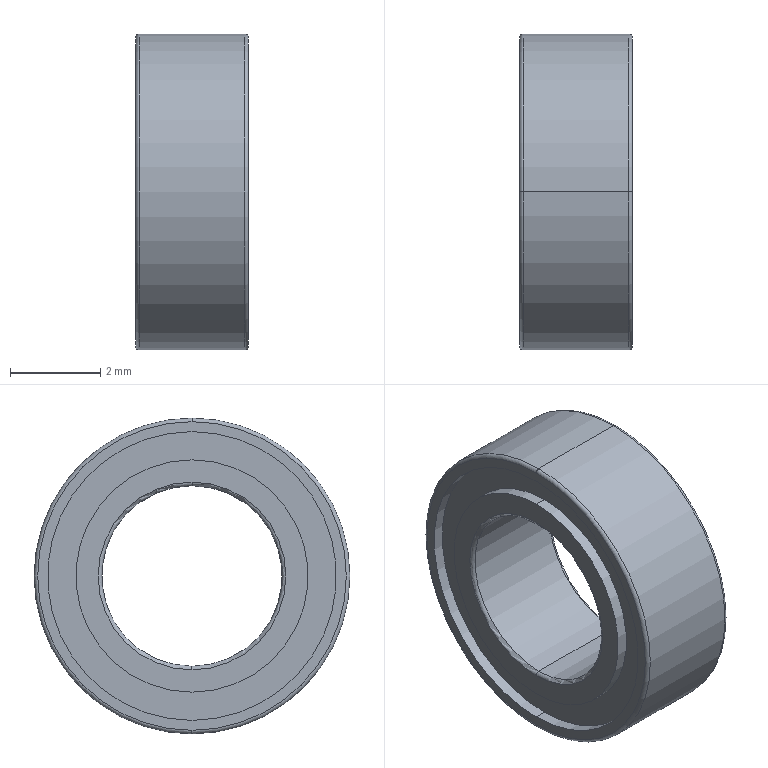Part | SolidWorks | features RefAxis 6, 3DProfileFeature 2, Revolution 1 | 1 solid | 26 faces | box 2.5 x 7 x 7 mm | volume 58.917 mm3 | cylinder 12 | torus 8 | plane 6 | commonest cylinder face diameters 5.15 x4 6.4 x4 4 x2 7 x2
STEP:
#1=CARTESIAN_POINT('',(2.42,0.,3.5));
#2=VERTEX_POINT('',#1);
#3=CARTESIAN_POINT('',(2.42,0.,-3.5));
#4=VERTEX_POINT('',#3);
#5=CARTESIAN_POINT('',(2.42,0.,0.));
#6=DIRECTION('',(-1.,0.,0.));
#7=DIRECTION('',(0.,0.,1.));
#8=AXIS2_PLACEMENT_3D('',#5,#6,#7);
#9=CIRCLE('',#8,3.5);
#10=EDGE_CURVE('',#2,#4,#9,.T.);
#11=ORIENTED_EDGE('',*,*,#10,.T.);
#12=CARTESIAN_POINT('',(0.08,0.,-3.5));
#13=VERTEX_POINT('',#12);
#14=CARTESIAN_POINT('',(2.42,0.,-3.5));
#15=DIRECTION('',(-1.,0.,0.));
#16=VECTOR('',#15,1000.);
#17=LINE('',#14,#16);
#18=EDGE_CURVE('',#4,#13,#17,.T.);
#19=ORIENTED_EDGE('',*,*,#18,.T.);
#20=CARTESIAN_POINT('',(0.08,0.,3.5));
#21=VERTEX_POINT('',#20);
#22=CARTESIAN_POINT('',(0.08,0.,0.));
#23=DIRECTION('',(-1.,0.,0.));
#24=DIRECTION('',(0.,0.,1.));
#25=AXIS2_PLACEMENT_3D('',#22,#23,#24);
#26=CIRCLE('',#25,3.5);
#27=EDGE_CURVE('',#21,#13,#26,.T.);
#28=ORIENTED_EDGE('',*,*,#27,.F.);
#29=CARTESIAN_POINT('',(2.42,0.,3.5));
#30=DIRECTION('',(-1.,0.,0.));
#31=VECTOR('',#30,1000.);
#32=LINE('',#29,#31);
#33=EDGE_CURVE('',#2,#21,#32,.T.);
#34=ORIENTED_EDGE('',*,*,#33,.F.);
#35=EDGE_LOOP('',(#11,#19,#28,#34));
#36=FACE_OUTER_BOUND('',#35,.T.);
#37=CARTESIAN_POINT('',(2.42,0.,0.));
#38=DIRECTION('',(-1.,0.,0.));
#39=DIRECTION('',(0.,0.,1.));
#40=AXIS2_PLACEMENT_3D('',#37,#38,#39);
#41=CYLINDRICAL_SURFACE('',#40,3.5);
#42=ADVANCED_FACE('',(#36),#41,.T.);
#43=CARTESIAN_POINT('',(2.5,0.,3.42));
#44=VERTEX_POINT('',#43);
#45=CARTESIAN_POINT('',(2.5,0.,-3.42));
#46=VERTEX_POINT('',#45);
#47=CARTESIAN_POINT('',(2.5,0.,0.));
#48=DIRECTION('',(-1.,0.,0.));
#49=DIRECTION('',(0.,0.,1.));
#50=AXIS2_PLACEMENT_3D('',#47,#48,#49);
#51=CIRCLE('',#50,3.42);
#52=EDGE_CURVE('',#44,#46,#51,.T.);
#53=ORIENTED_EDGE('',*,*,#52,.T.);
#54=CARTESIAN_POINT('',(2.42,0.,-3.42));
#55=DIRECTION('',(0.,1.,0.));
#56=DIRECTION('',(0.,0.,1.));
#57=AXIS2_PLACEMENT_3D('',#54,#55,#56);
#58=CIRCLE('',#57,0.08);
#59=EDGE_CURVE('',#46,#4,#58,.T.);
#60=ORIENTED_EDGE('',*,*,#59,.T.);
#61=ORIENTED_EDGE('',*,*,#10,.F.);
#62=CARTESIAN_POINT('',(2.42,0.,3.42));
#63=DIRECTION('',(0.,-1.,0.));
#64=DIRECTION('',(0.,0.,-1.));
#65=AXIS2_PLACEMENT_3D('',#62,#63,#64);
#66=CIRCLE('',#65,0.08);
#67=EDGE_CURVE('',#44,#2,#66,.T.);
#68=ORIENTED_EDGE('',*,*,#67,.F.);
#69=EDGE_LOOP('',(#53,#60,#61,#68));
#70=FACE_OUTER_BOUND('',#69,.T.);
#71=CARTESIAN_POINT('',(2.42,0.,0.));
#72=DIRECTION('',(-1.,0.,0.));
#73=DIRECTION('',(0.,0.,1.));
#74=AXIS2_PLACEMENT_3D('',#71,#72,#73);
#75=TOROIDAL_SURFACE('',#74,3.42,0.08);
#76=ADVANCED_FACE('',(#70),#75,.T.);
#77=CARTESIAN_POINT('',(2.5,0.,-3.2));
#78=VERTEX_POINT('',#77);
#79=CARTESIAN_POINT('',(2.5,0.,3.2));
#80=VERTEX_POINT('',#79);
#81=CARTESIAN_POINT('',(2.5,0.,0.));
#82=DIRECTION('',(-1.,0.,0.));
#83=DIRECTION('',(0.,0.,1.));
#84=AXIS2_PLACEMENT_3D('',#81,#82,#83);
#85=CIRCLE('',#84,3.2);
#86=EDGE_CURVE('',#78,#80,#85,.T.);
#87=ORIENTED_EDGE('',*,*,#86,.F.);
#88=CARTESIAN_POINT('',(2.245,0.,-3.2));
#89=VERTEX_POINT('',#88);
#90=CARTESIAN_POINT('',(2.42,0.,-3.2));
#91=DIRECTION('',(-1.,0.,0.));
#92=VECTOR('',#91,1000.);
#93=LINE('',#90,#92);
#94=EDGE_CURVE('',#78,#89,#93,.T.);
#95=ORIENTED_EDGE('',*,*,#94,.T.);
#96=CARTESIAN_POINT('',(2.245,0.,3.2));
#97=VERTEX_POINT('',#96);
#98=CARTESIAN_POINT('',(2.245,0.,0.));
#99=DIRECTION('',(-1.,0.,0.));
#100=DIRECTION('',(0.,0.,1.));
#101=AXIS2_PLACEMENT_3D('',#98,#99,#100);
#102=CIRCLE('',#101,3.2);
#103=EDGE_CURVE('',#89,#97,#102,.T.);
#104=ORIENTED_EDGE('',*,*,#103,.T.);
#105=CARTESIAN_POINT('',(2.42,0.,3.2));
#106=DIRECTION('',(-1.,0.,0.));
#107=VECTOR('',#106,1000.);
#108=LINE('',#105,#107);
#109=EDGE_CURVE('',#80,#97,#108,.T.);
#110=ORIENTED_EDGE('',*,*,#109,.F.);
#111=EDGE_LOOP('',(#87,#95,#104,#110));
#112=FACE_OUTER_BOUND('',#111,.T.);
#113=CARTESIAN_POINT('',(2.42,0.,0.));
#114=DIRECTION('',(-1.,0.,0.));
#115=DIRECTION('',(0.,0.,1.));
#116=AXIS2_PLACEMENT_3D('',#113,#114,#115);
#117=CYLINDRICAL_SURFACE('',#116,3.2);
#118=ADVANCED_FACE('',(#112),#117,.F.);
#119=CARTESIAN_POINT('',(2.5,0.,2.575));
#120=VERTEX_POINT('',#119);
#121=CARTESIAN_POINT('',(2.5,0.,-2.575));
#122=VERTEX_POINT('',#121);
#123=CARTESIAN_POINT('',(2.5,0.,0.));
#124=DIRECTION('',(-1.,0.,0.));
#125=DIRECTION('',(0.,0.,1.));
#126=AXIS2_PLACEMENT_3D('',#123,#124,#125);
#127=CIRCLE('',#126,2.575);
#128=EDGE_CURVE('',#120,#122,#127,.T.);
#129=ORIENTED_EDGE('',*,*,#128,.T.);
#130=CARTESIAN_POINT('',(2.245,0.,-2.575));
#131=VERTEX_POINT('',#130);
#132=CARTESIAN_POINT('',(2.42,0.,-2.575));
#133=DIRECTION('',(-1.,0.,0.));
#134=VECTOR('',#133,1000.);
#135=LINE('',#132,#134);
#136=EDGE_CURVE('',#122,#131,#135,.T.);
#137=ORIENTED_EDGE('',*,*,#136,.T.);
#138=CARTESIAN_POINT('',(2.245,0.,2.575));
#139=VERTEX_POINT('',#138);
#140=CARTESIAN_POINT('',(2.245,0.,0.));
#141=DIRECTION('',(-1.,0.,0.));
#142=DIRECTION('',(0.,0.,1.));
#143=AXIS2_PLACEMENT_3D('',#140,#141,#142);
#144=CIRCLE('',#143,2.575);
#145=EDGE_CURVE('',#139,#131,#144,.T.);
#146=ORIENTED_EDGE('',*,*,#145,.F.);
#147=CARTESIAN_POINT('',(2.42,0.,2.575));
#148=DIRECTION('',(-1.,0.,0.));
#149=VECTOR('',#148,1000.);
#150=LINE('',#147,#149);
#151=EDGE_CURVE('',#120,#139,#150,.T.);
#152=ORIENTED_EDGE('',*,*,#151,.F.);
#153=EDGE_LOOP('',(#129,#137,#146,#152));
#154=FACE_OUTER_BOUND('',#153,.T.);
#155=CARTESIAN_POINT('',(2.42,0.,0.));
#156=DIRECTION('',(-1.,0.,0.));
#157=DIRECTION('',(0.,0.,1.));
#158=AXIS2_PLACEMENT_3D('',#155,#156,#157);
#159=CYLINDRICAL_SURFACE('',#158,2.575);
#160=ADVANCED_FACE('',(#154),#159,.T.);
#161=CARTESIAN_POINT('',(2.42,0.,2.));
#162=VERTEX_POINT('',#161);
#163=CARTESIAN_POINT('',(2.42,0.,-2.));
#164=VERTEX_POINT('',#163);
#165=CARTESIAN_POINT('',(2.42,0.,0.));
#166=DIRECTION('',(-1.,0.,0.));
#167=DIRECTION('',(0.,0.,1.));
#168=AXIS2_PLACEMENT_3D('',#165,#166,#167);
#169=CIRCLE('',#168,2.);
#170=EDGE_CURVE('',#162,#164,#169,.T.);
#171=ORIENTED_EDGE('',*,*,#170,.T.);
#172=CARTESIAN_POINT('',(2.5,0.,-2.08));
#173=VERTEX_POINT('',#172);
#174=CARTESIAN_POINT('',(2.42,0.,-2.08));
#175=DIRECTION('',(0.,1.,0.));
#176=DIRECTION('',(0.,0.,1.));
#177=AXIS2_PLACEMENT_3D('',#174,#175,#176);
#178=CIRCLE('',#177,0.08);
#179=EDGE_CURVE('',#164,#173,#178,.T.);
#180=ORIENTED_EDGE('',*,*,#179,.T.);
#181=CARTESIAN_POINT('',(2.5,0.,2.08));
#182=VERTEX_POINT('',#181);
#183=CARTESIAN_POINT('',(2.5,0.,0.));
#184=DIRECTION('',(-1.,0.,0.));
#185=DIRECTION('',(0.,0.,1.));
#186=AXIS2_PLACEMENT_3D('',#183,#184,#185);
#187=CIRCLE('',#186,2.08);
#188=EDGE_CURVE('',#182,#173,#187,.T.);
#189=ORIENTED_EDGE('',*,*,#188,.F.);
#190=CARTESIAN_POINT('',(2.42,0.,2.08));
#191=DIRECTION('',(0.,-1.,0.));
#192=DIRECTION('',(0.,0.,-1.));
#193=AXIS2_PLACEMENT_3D('',#190,#191,#192);
#194=CIRCLE('',#193,0.08);
#195=EDGE_CURVE('',#162,#182,#194,.T.);
#196=ORIENTED_EDGE('',*,*,#195,.F.);
#197=EDGE_LOOP('',(#171,#180,#189,#196));
#198=FACE_OUTER_BOUND('',#197,.T.);
#199=CARTESIAN_POINT('',(2.42,0.,0.));
#200=DIRECTION('',(-1.,0.,0.));
#201=DIRECTION('',(0.,0.,1.));
#202=AXIS2_PLACEMENT_3D('',#199,#200,#201);
#203=TOROIDAL_SURFACE('',#202,2.08,0.08);
#204=ADVANCED_FACE('',(#198),#203,.T.);
#205=CARTESIAN_POINT('',(2.42,0.,0.));
#206=DIRECTION('',(-1.,0.,0.));
#207=DIRECTION('',(0.,0.,1.));
#208=AXIS2_PLACEMENT_3D('',#205,#206,#207);
#209=CIRCLE('',#208,2.);
#210=EDGE_CURVE('',#164,#162,#209,.T.);
#211=ORIENTED_EDGE('',*,*,#210,.F.);
#212=CARTESIAN_POINT('',(0.08,0.,-2.));
#213=VERTEX_POINT('',#212);
#214=CARTESIAN_POINT('',(2.42,0.,-2.));
#215=DIRECTION('',(-1.,0.,0.));
#216=VECTOR('',#215,1000.);
#217=LINE('',#214,#216);
#218=EDGE_CURVE('',#164,#213,#217,.T.);
#219=ORIENTED_EDGE('',*,*,#218,.T.);
#220=CARTESIAN_POINT('',(0.08,0.,2.));
#221=VERTEX_POINT('',#220);
#222=CARTESIAN_POINT('',(0.08,0.,0.));
#223=DIRECTION('',(-1.,0.,0.));
#224=DIRECTION('',(0.,0.,1.));
#225=AXIS2_PLACEMENT_3D('',#222,#223,#224);
#226=CIRCLE('',#225,2.);
#227=EDGE_CURVE('',#213,#221,#226,.T.);
#228=ORIENTED_EDGE('',*,*,#227,.T.);
#229=CARTESIAN_POINT('',(2.42,0.,2.));
#230=DIRECTION('',(-1.,0.,0.));
#231=VECTOR('',#230,1000.);
#232=LINE('',#229,#231);
#233=EDGE_CURVE('',#162,#221,#232,.T.);
#234=ORIENTED_EDGE('',*,*,#233,.F.);
#235=EDGE_LOOP('',(#211,#219,#228,#234));
#236=FACE_OUTER_BOUND('',#235,.T.);
#237=CARTESIAN_POINT('',(2.42,0.,0.));
#238=DIRECTION('',(-1.,0.,0.));
#239=DIRECTION('',(0.,0.,1.));
#240=AXIS2_PLACEMENT_3D('',#237,#238,#239);
#241=CYLINDRICAL_SURFACE('',#240,2.);
#242=ADVANCED_FACE('',(#236),#241,.F.);
#243=CARTESIAN_POINT('',(0.,0.,2.08));
#244=VERTEX_POINT('',#243);
#245=CARTESIAN_POINT('',(0.,0.,-2.08));
#246=VERTEX_POINT('',#245);
#247=CARTESIAN_POINT('',(0.,0.,0.));
#248=DIRECTION('',(-1.,0.,0.));
#249=DIRECTION('',(0.,0.,1.));
#250=AXIS2_PLACEMENT_3D('',#247,#248,#249);
#251=CIRCLE('',#250,2.08);
#252=EDGE_CURVE('',#244,#246,#251,.T.);
#253=ORIENTED_EDGE('',*,*,#252,.T.);
#254=CARTESIAN_POINT('',(0.08,0.,-2.08));
#255=DIRECTION('',(0.,1.,0.));
#256=DIRECTION('',(0.,0.,1.));
#257=AXIS2_PLACEMENT_3D('',#254,#255,#256);
#258=CIRCLE('',#257,0.08);
#259=EDGE_CURVE('',#246,#213,#258,.T.);
#260=ORIENTED_EDGE('',*,*,#259,.T.);
#261=CARTESIAN_POINT('',(0.08,0.,0.));
#262=DIRECTION('',(-1.,0.,0.));
#263=DIRECTION('',(0.,0.,1.));
#264=AXIS2_PLACEMENT_3D('',#261,#262,#263);
#265=CIRCLE('',#264,2.);
#266=EDGE_CURVE('',#221,#213,#265,.T.);
#267=ORIENTED_EDGE('',*,*,#266,.F.);
#268=CARTESIAN_POINT('',(0.08,0.,2.08));
#269=DIRECTION('',(0.,-1.,0.));
#270=DIRECTION('',(0.,0.,-1.));
#271=AXIS2_PLACEMENT_3D('',#268,#269,#270);
#272=CIRCLE('',#271,0.08);
#273=EDGE_CURVE('',#244,#221,#272,.T.);
#274=ORIENTED_EDGE('',*,*,#273,.F.);
#275=EDGE_LOOP('',(#253,#260,#267,#274));
#276=FACE_OUTER_BOUND('',#275,.T.);
#277=CARTESIAN_POINT('',(0.08,0.,0.));
#278=DIRECTION('',(-1.,0.,0.));
#279=DIRECTION('',(0.,0.,1.));
#280=AXIS2_PLACEMENT_3D('',#277,#278,#279);
#281=TOROIDAL_SURFACE('',#280,2.08,0.08);
#282=ADVANCED_FACE('',(#276),#281,.T.);
#283=CARTESIAN_POINT('',(0.255,0.,2.575));
#284=VERTEX_POINT('',#283);
#285=CARTESIAN_POINT('',(0.255,0.,-2.575));
#286=VERTEX_POINT('',#285);
#287=CARTESIAN_POINT('',(0.255,0.,0.));
#288=DIRECTION('',(-1.,0.,0.));
#289=DIRECTION('',(0.,0.,1.));
#290=AXIS2_PLACEMENT_3D('',#287,#288,#289);
#291=CIRCLE('',#290,2.575);
#292=EDGE_CURVE('',#284,#286,#291,.T.);
#293=ORIENTED_EDGE('',*,*,#292,.T.);
#294=CARTESIAN_POINT('',(0.,0.,-2.575));
#295=VERTEX_POINT('',#294);
#296=CARTESIAN_POINT('',(2.42,0.,-2.575));
#297=DIRECTION('',(-1.,0.,0.));
#298=VECTOR('',#297,1000.);
#299=LINE('',#296,#298);
#300=EDGE_CURVE('',#286,#295,#299,.T.);
#301=ORIENTED_EDGE('',*,*,#300,.T.);
#302=CARTESIAN_POINT('',(0.,0.,2.575));
#303=VERTEX_POINT('',#302);
#304=CARTESIAN_POINT('',(0.,0.,0.));
#305=DIRECTION('',(-1.,0.,0.));
#306=DIRECTION('',(0.,0.,1.));
#307=AXIS2_PLACEMENT_3D('',#304,#305,#306);
#308=CIRCLE('',#307,2.575);
#309=EDGE_CURVE('',#303,#295,#308,.T.);
#310=ORIENTED_EDGE('',*,*,#309,.F.);
#311=CARTESIAN_POINT('',(2.42,0.,2.575));
#312=DIRECTION('',(-1.,0.,0.));
#313=VECTOR('',#312,1000.);
#314=LINE('',#311,#313);
#315=EDGE_CURVE('',#284,#303,#314,.T.);
#316=ORIENTED_EDGE('',*,*,#315,.F.);
#317=EDGE_LOOP('',(#293,#301,#310,#316));
#318=FACE_OUTER_BOUND('',#317,.T.);
#319=CARTESIAN_POINT('',(2.42,0.,0.));
#320=DIRECTION('',(-1.,0.,0.));
#321=DIRECTION('',(0.,0.,1.));
#322=AXIS2_PLACEMENT_3D('',#319,#320,#321);
#323=CYLINDRICAL_SURFACE('',#322,2.575);
#324=ADVANCED_FACE('',(#318),#323,.T.);
#325=CARTESIAN_POINT('',(0.255,0.,-3.2));
#326=VERTEX_POINT('',#325);
#327=CARTESIAN_POINT('',(0.255,0.,3.2));
#328=VERTEX_POINT('',#327);
#329=CARTESIAN_POINT('',(0.255,0.,0.));
#330=DIRECTION('',(-1.,0.,0.));
#331=DIRECTION('',(0.,0.,1.));
#332=AXIS2_PLACEMENT_3D('',#329,#330,#331);
#333=CIRCLE('',#332,3.2);
#334=EDGE_CURVE('',#326,#328,#333,.T.);
#335=ORIENTED_EDGE('',*,*,#334,.F.);
#336=CARTESIAN_POINT('',(0.,0.,-3.2));
#337=VERTEX_POINT('',#336);
#338=CARTESIAN_POINT('',(2.42,0.,-3.2));
#339=DIRECTION('',(-1.,0.,0.));
#340=VECTOR('',#339,1000.);
#341=LINE('',#338,#340);
#342=EDGE_CURVE('',#326,#337,#341,.T.);
#343=ORIENTED_EDGE('',*,*,#342,.T.);
#344=CARTESIAN_POINT('',(0.,0.,3.2));
#345=VERTEX_POINT('',#344);
#346=CARTESIAN_POINT('',(0.,0.,0.));
#347=DIRECTION('',(-1.,0.,0.));
#348=DIRECTION('',(0.,0.,1.));
#349=AXIS2_PLACEMENT_3D('',#346,#347,#348);
#350=CIRCLE('',#349,3.2);
#351=EDGE_CURVE('',#337,#345,#350,.T.);
#352=ORIENTED_EDGE('',*,*,#351,.T.);
#353=CARTESIAN_POINT('',(2.42,0.,3.2));
#354=DIRECTION('',(-1.,0.,0.));
#355=VECTOR('',#354,1000.);
#356=LINE('',#353,#355);
#357=EDGE_CURVE('',#328,#345,#356,.T.);
#358=ORIENTED_EDGE('',*,*,#357,.F.);
#359=EDGE_LOOP('',(#335,#343,#352,#358));
#360=FACE_OUTER_BOUND('',#359,.T.);
#361=CARTESIAN_POINT('',(2.42,0.,0.));
#362=DIRECTION('',(-1.,0.,0.));
#363=DIRECTION('',(0.,0.,1.));
#364=AXIS2_PLACEMENT_3D('',#361,#362,#363);
#365=CYLINDRICAL_SURFACE('',#364,3.2);
#366=ADVANCED_FACE('',(#360),#365,.F.);
#367=ORIENTED_EDGE('',*,*,#27,.T.);
#368=CARTESIAN_POINT('',(0.,0.,-3.42));
#369=VERTEX_POINT('',#368);
#370=CARTESIAN_POINT('',(0.08,0.,-3.42));
#371=DIRECTION('',(0.,1.,0.));
#372=DIRECTION('',(0.,0.,1.));
#373=AXIS2_PLACEMENT_3D('',#370,#371,#372);
#374=CIRCLE('',#373,0.08);
#375=EDGE_CURVE('',#13,#369,#374,.T.);
#376=ORIENTED_EDGE('',*,*,#375,.T.);
#377=CARTESIAN_POINT('',(0.,0.,3.42));
#378=VERTEX_POINT('',#377);
#379=CARTESIAN_POINT('',(0.,0.,0.));
#380=DIRECTION('',(-1.,0.,0.));
#381=DIRECTION('',(0.,0.,1.));
#382=AXIS2_PLACEMENT_3D('',#379,#380,#381);
#383=CIRCLE('',#382,3.42);
#384=EDGE_CURVE('',#378,#369,#383,.T.);
#385=ORIENTED_EDGE('',*,*,#384,.F.);
#386=CARTESIAN_POINT('',(0.08,0.,3.42));
#387=DIRECTION('',(0.,-1.,0.));
#388=DIRECTION('',(0.,0.,-1.));
#389=AXIS2_PLACEMENT_3D('',#386,#387,#388);
#390=CIRCLE('',#389,0.08);
#391=EDGE_CURVE('',#21,#378,#390,.T.);
#392=ORIENTED_EDGE('',*,*,#391,.F.);
#393=EDGE_LOOP('',(#367,#376,#385,#392));
#394=FACE_OUTER_BOUND('',#393,.T.);
#395=CARTESIAN_POINT('',(0.08,0.,0.));
#396=DIRECTION('',(-1.,0.,0.));
#397=DIRECTION('',(0.,0.,1.));
#398=AXIS2_PLACEMENT_3D('',#395,#396,#397);
#399=TOROIDAL_SURFACE('',#398,3.42,0.08);
#400=ADVANCED_FACE('',(#394),#399,.T.);
#401=ORIENTED_EDGE('',*,*,#375,.F.);
#402=CARTESIAN_POINT('',(0.08,0.,0.));
#403=DIRECTION('',(-1.,0.,0.));
#404=DIRECTION('',(0.,0.,1.));
#405=AXIS2_PLACEMENT_3D('',#402,#403,#404);
#406=CIRCLE('',#405,3.5);
#407=EDGE_CURVE('',#13,#21,#406,.T.);
#408=ORIENTED_EDGE('',*,*,#407,.T.);
#409=ORIENTED_EDGE('',*,*,#391,.T.);
#410=CARTESIAN_POINT('',(0.,0.,0.));
#411=DIRECTION('',(-1.,0.,0.));
#412=DIRECTION('',(0.,0.,1.));
#413=AXIS2_PLACEMENT_3D('',#410,#411,#412);
#414=CIRCLE('',#413,3.42);
#415=EDGE_CURVE('',#369,#378,#414,.T.);
#416=ORIENTED_EDGE('',*,*,#415,.F.);
#417=EDGE_LOOP('',(#401,#408,#409,#416));
#418=FACE_OUTER_BOUND('',#417,.T.);
#419=CARTESIAN_POINT('',(0.08,0.,0.));
#420=DIRECTION('',(-1.,0.,0.));
#421=DIRECTION('',(0.,0.,1.));
#422=AXIS2_PLACEMENT_3D('',#419,#420,#421);
#423=TOROIDAL_SURFACE('',#422,3.42,0.08);
#424=ADVANCED_FACE('',(#418),#423,.T.);
#425=CARTESIAN_POINT('',(0.,0.,0.));
#426=DIRECTION('',(-1.,0.,0.));
#427=DIRECTION('',(0.,0.,1.));
#428=AXIS2_PLACEMENT_3D('',#425,#426,#427);
#429=CIRCLE('',#428,3.2);
#430=EDGE_CURVE('',#345,#337,#429,.T.);
#431=ORIENTED_EDGE('',*,*,#430,.F.);
#432=ORIENTED_EDGE('',*,*,#351,.F.);
#433=EDGE_LOOP('',(#431,#432));
#434=FACE_BOUND('',#433,.T.);
#435=ORIENTED_EDGE('',*,*,#384,.T.);
#436=ORIENTED_EDGE('',*,*,#415,.T.);
#437=EDGE_LOOP('',(#435,#436));
#438=FACE_OUTER_BOUND('',#437,.T.);
#439=CARTESIAN_POINT('',(0.,3.42,0.));
#440=DIRECTION('',(1.,0.,0.));
#441=DIRECTION('',(0.,0.,-1.));
#442=AXIS2_PLACEMENT_3D('',#439,#440,#441);
#443=PLANE('',#442);
#444=ADVANCED_FACE('',(#434,#438),#443,.F.);
#445=ORIENTED_EDGE('',*,*,#342,.F.);
#446=CARTESIAN_POINT('',(0.255,0.,0.));
#447=DIRECTION('',(-1.,0.,0.));
#448=DIRECTION('',(0.,0.,1.));
#449=AXIS2_PLACEMENT_3D('',#446,#447,#448);
#450=CIRCLE('',#449,3.2);
#451=EDGE_CURVE('',#328,#326,#450,.T.);
#452=ORIENTED_EDGE('',*,*,#451,.F.);
#453=ORIENTED_EDGE('',*,*,#357,.T.);
#454=ORIENTED_EDGE('',*,*,#430,.T.);
#455=EDGE_LOOP('',(#445,#452,#453,#454));
#456=FACE_OUTER_BOUND('',#455,.T.);
#457=CARTESIAN_POINT('',(2.42,0.,0.));
#458=DIRECTION('',(-1.,0.,0.));
#459=DIRECTION('',(0.,0.,1.));
#460=AXIS2_PLACEMENT_3D('',#457,#458,#459);
#461=CYLINDRICAL_SURFACE('',#460,3.2);
#462=ADVANCED_FACE('',(#456),#461,.F.);
#463=ORIENTED_EDGE('',*,*,#292,.F.);
#464=CARTESIAN_POINT('',(0.255,0.,0.));
#465=DIRECTION('',(-1.,0.,0.));
#466=DIRECTION('',(0.,0.,1.));
#467=AXIS2_PLACEMENT_3D('',#464,#465,#466);
#468=CIRCLE('',#467,2.575);
#469=EDGE_CURVE('',#286,#284,#468,.T.);
#470=ORIENTED_EDGE('',*,*,#469,.F.);
#471=EDGE_LOOP('',(#463,#470));
#472=FACE_BOUND('',#471,.T.);
#473=ORIENTED_EDGE('',*,*,#451,.T.);
#474=ORIENTED_EDGE('',*,*,#334,.T.);
#475=EDGE_LOOP('',(#473,#474));
#476=FACE_OUTER_BOUND('',#475,.T.);
#477=CARTESIAN_POINT('',(0.255,3.2,0.));
#478=DIRECTION('',(1.,0.,0.));
#479=DIRECTION('',(0.,0.,-1.));
#480=AXIS2_PLACEMENT_3D('',#477,#478,#479);
#481=PLANE('',#480);
#482=ADVANCED_FACE('',(#472,#476),#481,.F.);
#483=ORIENTED_EDGE('',*,*,#300,.F.);
#484=ORIENTED_EDGE('',*,*,#469,.T.);
#485=ORIENTED_EDGE('',*,*,#315,.T.);
#486=CARTESIAN_POINT('',(0.,0.,0.));
#487=DIRECTION('',(-1.,0.,0.));
#488=DIRECTION('',(0.,0.,1.));
#489=AXIS2_PLACEMENT_3D('',#486,#487,#488);
#490=CIRCLE('',#489,2.575);
#491=EDGE_CURVE('',#295,#303,#490,.T.);
#492=ORIENTED_EDGE('',*,*,#491,.F.);
#493=EDGE_LOOP('',(#483,#484,#485,#492));
#494=FACE_OUTER_BOUND('',#493,.T.);
#495=CARTESIAN_POINT('',(2.42,0.,0.));
#496=DIRECTION('',(-1.,0.,0.));
#497=DIRECTION('',(0.,0.,1.));
#498=AXIS2_PLACEMENT_3D('',#495,#496,#497);
#499=CYLINDRICAL_SURFACE('',#498,2.575);
#500=ADVANCED_FACE('',(#494),#499,.T.);
#501=ORIENTED_EDGE('',*,*,#252,.F.);
#502=CARTESIAN_POINT('',(0.,0.,0.));
#503=DIRECTION('',(-1.,0.,0.));
#504=DIRECTION('',(0.,0.,1.));
#505=AXIS2_PLACEMENT_3D('',#502,#503,#504);
#506=CIRCLE('',#505,2.08);
#507=EDGE_CURVE('',#246,#244,#506,.T.);
#508=ORIENTED_EDGE('',*,*,#507,.F.);
#509=EDGE_LOOP('',(#501,#508));
#510=FACE_BOUND('',#509,.T.);
#511=ORIENTED_EDGE('',*,*,#309,.T.);
#512=ORIENTED_EDGE('',*,*,#491,.T.);
#513=EDGE_LOOP('',(#511,#512));
#514=FACE_OUTER_BOUND('',#513,.T.);
#515=CARTESIAN_POINT('',(0.,2.575,0.));
#516=DIRECTION('',(1.,0.,0.));
#517=DIRECTION('',(0.,0.,-1.));
#518=AXIS2_PLACEMENT_3D('',#515,#516,#517);
#519=PLANE('',#518);
#520=ADVANCED_FACE('',(#510,#514),#519,.F.);
#521=ORIENTED_EDGE('',*,*,#259,.F.);
#522=ORIENTED_EDGE('',*,*,#507,.T.);
#523=ORIENTED_EDGE('',*,*,#273,.T.);
#524=ORIENTED_EDGE('',*,*,#227,.F.);
#525=EDGE_LOOP('',(#521,#522,#523,#524));
#526=FACE_OUTER_BOUND('',#525,.T.);
#527=CARTESIAN_POINT('',(0.08,0.,0.));
#528=DIRECTION('',(-1.,0.,0.));
#529=DIRECTION('',(0.,0.,1.));
#530=AXIS2_PLACEMENT_3D('',#527,#528,#529);
#531=TOROIDAL_SURFACE('',#530,2.08,0.08);
#532=ADVANCED_FACE('',(#526),#531,.T.);
#533=ORIENTED_EDGE('',*,*,#218,.F.);
#534=ORIENTED_EDGE('',*,*,#170,.F.);
#535=ORIENTED_EDGE('',*,*,#233,.T.);
#536=ORIENTED_EDGE('',*,*,#266,.T.);
#537=EDGE_LOOP('',(#533,#534,#535,#536));
#538=FACE_OUTER_BOUND('',#537,.T.);
#539=CARTESIAN_POINT('',(2.42,0.,0.));
#540=DIRECTION('',(-1.,0.,0.));
#541=DIRECTION('',(0.,0.,1.));
#542=AXIS2_PLACEMENT_3D('',#539,#540,#541);
#543=CYLINDRICAL_SURFACE('',#542,2.);
#544=ADVANCED_FACE('',(#538),#543,.F.);
#545=ORIENTED_EDGE('',*,*,#179,.F.);
#546=ORIENTED_EDGE('',*,*,#210,.T.);
#547=ORIENTED_EDGE('',*,*,#195,.T.);
#548=CARTESIAN_POINT('',(2.5,0.,0.));
#549=DIRECTION('',(-1.,0.,0.));
#550=DIRECTION('',(0.,0.,1.));
#551=AXIS2_PLACEMENT_3D('',#548,#549,#550);
#552=CIRCLE('',#551,2.08);
#553=EDGE_CURVE('',#173,#182,#552,.T.);
#554=ORIENTED_EDGE('',*,*,#553,.F.);
#555=EDGE_LOOP('',(#545,#546,#547,#554));
#556=FACE_OUTER_BOUND('',#555,.T.);
#557=CARTESIAN_POINT('',(2.42,0.,0.));
#558=DIRECTION('',(-1.,0.,0.));
#559=DIRECTION('',(0.,0.,1.));
#560=AXIS2_PLACEMENT_3D('',#557,#558,#559);
#561=TOROIDAL_SURFACE('',#560,2.08,0.08);
#562=ADVANCED_FACE('',(#556),#561,.T.);
#563=ORIENTED_EDGE('',*,*,#128,.F.);
#564=CARTESIAN_POINT('',(2.5,0.,0.));
#565=DIRECTION('',(-1.,0.,0.));
#566=DIRECTION('',(0.,0.,1.));
#567=AXIS2_PLACEMENT_3D('',#564,#565,#566);
#568=CIRCLE('',#567,2.575);
#569=EDGE_CURVE('',#122,#120,#568,.T.);
#570=ORIENTED_EDGE('',*,*,#569,.F.);
#571=EDGE_LOOP('',(#563,#570));
#572=FACE_OUTER_BOUND('',#571,.T.);
#573=ORIENTED_EDGE('',*,*,#188,.T.);
#574=ORIENTED_EDGE('',*,*,#553,.T.);
#575=EDGE_LOOP('',(#573,#574));
#576=FACE_BOUND('',#575,.T.);
#577=CARTESIAN_POINT('',(2.5,2.08,0.));
#578=DIRECTION('',(-1.,0.,0.));
#579=DIRECTION('',(0.,0.,1.));
#580=AXIS2_PLACEMENT_3D('',#577,#578,#579);
#581=PLANE('',#580);
#582=ADVANCED_FACE('',(#572,#576),#581,.F.);
#583=ORIENTED_EDGE('',*,*,#136,.F.);
#584=ORIENTED_EDGE('',*,*,#569,.T.);
#585=ORIENTED_EDGE('',*,*,#151,.T.);
#586=CARTESIAN_POINT('',(2.245,0.,0.));
#587=DIRECTION('',(-1.,0.,0.));
#588=DIRECTION('',(0.,0.,1.));
#589=AXIS2_PLACEMENT_3D('',#586,#587,#588);
#590=CIRCLE('',#589,2.575);
#591=EDGE_CURVE('',#131,#139,#590,.T.);
#592=ORIENTED_EDGE('',*,*,#591,.F.);
#593=EDGE_LOOP('',(#583,#584,#585,#592));
#594=FACE_OUTER_BOUND('',#593,.T.);
#595=CARTESIAN_POINT('',(2.42,0.,0.));
#596=DIRECTION('',(-1.,0.,0.));
#597=DIRECTION('',(0.,0.,1.));
#598=AXIS2_PLACEMENT_3D('',#595,#596,#597);
#599=CYLINDRICAL_SURFACE('',#598,2.575);
#600=ADVANCED_FACE('',(#594),#599,.T.);
#601=CARTESIAN_POINT('',(2.245,0.,0.));
#602=DIRECTION('',(-1.,0.,0.));
#603=DIRECTION('',(0.,0.,1.));
#604=AXIS2_PLACEMENT_3D('',#601,#602,#603);
#605=CIRCLE('',#604,3.2);
#606=EDGE_CURVE('',#97,#89,#605,.T.);
#607=ORIENTED_EDGE('',*,*,#606,.F.);
#608=ORIENTED_EDGE('',*,*,#103,.F.);
#609=EDGE_LOOP('',(#607,#608));
#610=FACE_OUTER_BOUND('',#609,.T.);
#611=ORIENTED_EDGE('',*,*,#145,.T.);
#612=ORIENTED_EDGE('',*,*,#591,.T.);
#613=EDGE_LOOP('',(#611,#612));
#614=FACE_BOUND('',#613,.T.);
#615=CARTESIAN_POINT('',(2.245,2.575,0.));
#616=DIRECTION('',(-1.,0.,0.));
#617=DIRECTION('',(0.,0.,1.));
#618=AXIS2_PLACEMENT_3D('',#615,#616,#617);
#619=PLANE('',#618);
#620=ADVANCED_FACE('',(#610,#614),#619,.F.);
#621=ORIENTED_EDGE('',*,*,#94,.F.);
#622=CARTESIAN_POINT('',(2.5,0.,0.));
#623=DIRECTION('',(-1.,0.,0.));
#624=DIRECTION('',(0.,0.,1.));
#625=AXIS2_PLACEMENT_3D('',#622,#623,#624);
#626=CIRCLE('',#625,3.2);
#627=EDGE_CURVE('',#80,#78,#626,.T.);
#628=ORIENTED_EDGE('',*,*,#627,.F.);
#629=ORIENTED_EDGE('',*,*,#109,.T.);
#630=ORIENTED_EDGE('',*,*,#606,.T.);
#631=EDGE_LOOP('',(#621,#628,#629,#630));
#632=FACE_OUTER_BOUND('',#631,.T.);
#633=CARTESIAN_POINT('',(2.42,0.,0.));
#634=DIRECTION('',(-1.,0.,0.));
#635=DIRECTION('',(0.,0.,1.));
#636=AXIS2_PLACEMENT_3D('',#633,#634,#635);
#637=CYLINDRICAL_SURFACE('',#636,3.2);
#638=ADVANCED_FACE('',(#632),#637,.F.);
#639=ORIENTED_EDGE('',*,*,#52,.F.);
#640=CARTESIAN_POINT('',(2.5,0.,0.));
#641=DIRECTION('',(-1.,0.,0.));
#642=DIRECTION('',(0.,0.,1.));
#643=AXIS2_PLACEMENT_3D('',#640,#641,#642);
#644=CIRCLE('',#643,3.42);
#645=EDGE_CURVE('',#46,#44,#644,.T.);
#646=ORIENTED_EDGE('',*,*,#645,.F.);
#647=EDGE_LOOP('',(#639,#646));
#648=FACE_OUTER_BOUND('',#647,.T.);
#649=ORIENTED_EDGE('',*,*,#627,.T.);
#650=ORIENTED_EDGE('',*,*,#86,.T.);
#651=EDGE_LOOP('',(#649,#650));
#652=FACE_BOUND('',#651,.T.);
#653=CARTESIAN_POINT('',(2.5,3.2,0.));
#654=DIRECTION('',(-1.,0.,0.));
#655=DIRECTION('',(0.,0.,1.));
#656=AXIS2_PLACEMENT_3D('',#653,#654,#655);
#657=PLANE('',#656);
#658=ADVANCED_FACE('',(#648,#652),#657,.F.);
#659=ORIENTED_EDGE('',*,*,#59,.F.);
#660=ORIENTED_EDGE('',*,*,#645,.T.);
#661=ORIENTED_EDGE('',*,*,#67,.T.);
#662=CARTESIAN_POINT('',(2.42,0.,0.));
#663=DIRECTION('',(-1.,0.,0.));
#664=DIRECTION('',(0.,0.,1.));
#665=AXIS2_PLACEMENT_3D('',#662,#663,#664);
#666=CIRCLE('',#665,3.5);
#667=EDGE_CURVE('',#4,#2,#666,.T.);
#668=ORIENTED_EDGE('',*,*,#667,.F.);
#669=EDGE_LOOP('',(#659,#660,#661,#668));
#670=FACE_OUTER_BOUND('',#669,.T.);
#671=CARTESIAN_POINT('',(2.42,0.,0.));
#672=DIRECTION('',(-1.,0.,0.));
#673=DIRECTION('',(0.,0.,1.));
#674=AXIS2_PLACEMENT_3D('',#671,#672,#673);
#675=TOROIDAL_SURFACE('',#674,3.42,0.08);
#676=ADVANCED_FACE('',(#670),#675,.T.);
#677=ORIENTED_EDGE('',*,*,#18,.F.);
#678=ORIENTED_EDGE('',*,*,#667,.T.);
#679=ORIENTED_EDGE('',*,*,#33,.T.);
#680=ORIENTED_EDGE('',*,*,#407,.F.);
#681=EDGE_LOOP('',(#677,#678,#679,#680));
#682=FACE_OUTER_BOUND('',#681,.T.);
#683=CARTESIAN_POINT('',(2.42,0.,0.));
#684=DIRECTION('',(-1.,0.,0.));
#685=DIRECTION('',(0.,0.,1.));
#686=AXIS2_PLACEMENT_3D('',#683,#684,#685);
#687=CYLINDRICAL_SURFACE('',#686,3.5);
#688=ADVANCED_FACE('',(#682),#687,.T.);
#689=CLOSED_SHELL('',(#42,#76,#118,#160,#204,#242,#282,#324,#366,#400,#424,#444,#462,#482,#500,#520,#532,#544,#562,#582,#600,#620,#638,#658,#676,#688));
#690=MANIFOLD_SOLID_BREP('',#689);
#691=CARTESIAN_POINT('',(0.,0.,0.));
#692=DIRECTION('',(0.,0.,1.));
#693=DIRECTION('',(1.,0.,0.));
#694=AXIS2_PLACEMENT_3D('',#691,#692,#693);
#695=(LENGTH_UNIT()NAMED_UNIT(*)SI_UNIT(.MILLI.,.METRE.));
#696=UNCERTAINTY_MEASURE_WITH_UNIT(LENGTH_MEASURE(0.00001),#695,'','');
#697=(NAMED_UNIT(*)PLANE_ANGLE_UNIT()SI_UNIT($,.RADIAN.));
#698=(NAMED_UNIT(*)SI_UNIT($,.STERADIAN.)SOLID_ANGLE_UNIT());
#699=(GEOMETRIC_REPRESENTATION_CONTEXT(3)GLOBAL_UNCERTAINTY_ASSIGNED_CONTEXT((#696))GLOBAL_UNIT_ASSIGNED_CONTEXT((#695,#697,#698))REPRESENTATION_CONTEXT('',''));
#700=ADVANCED_BREP_SHAPE_REPRESENTATION('',(#690,#694),#699);